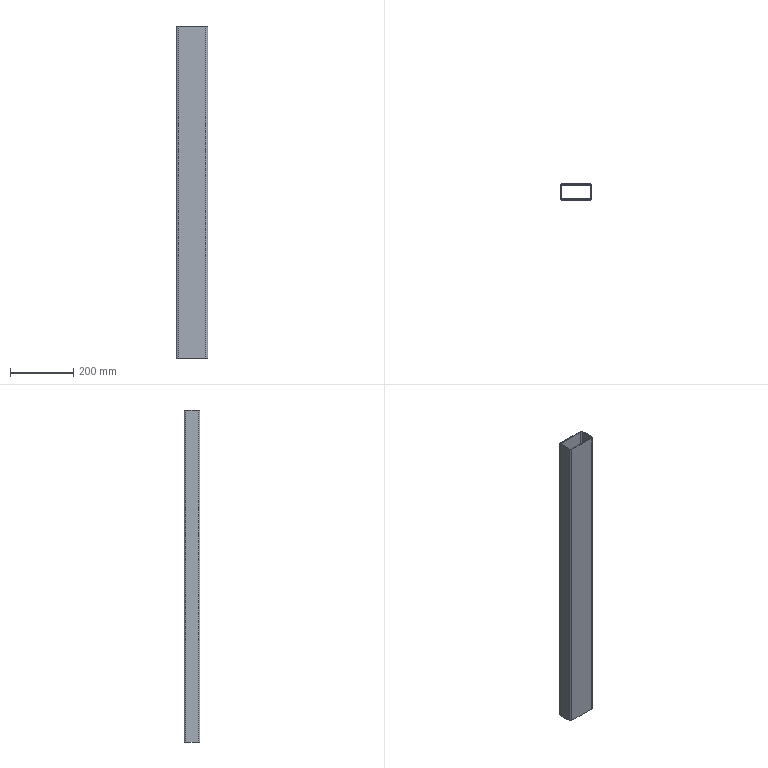Part | SolidWorks | features BaseBody 1 | 1 solid | 18 faces | box 100 x 50 x 1046 mm | volume 879501 mm3 | plane 10 | cylinder 8 | commonest cylinder face diameters 6 x4 12 x4
STEP:
#1=CARTESIAN_POINT('',(-44.,-22.,0.));
#2=VERTEX_POINT('',#1);
#3=CARTESIAN_POINT('',(44.,-22.,0.));
#4=VERTEX_POINT('',#3);
#5=CARTESIAN_POINT('',(44.,-22.,0.));
#6=DIRECTION('',(1.,0.,0.));
#7=VECTOR('',#6,1000.);
#8=LINE('',#5,#7);
#9=EDGE_CURVE('',#2,#4,#8,.T.);
#10=ORIENTED_EDGE('',*,*,#9,.F.);
#11=CARTESIAN_POINT('',(-44.,-22.,1046.));
#12=VERTEX_POINT('',#11);
#13=CARTESIAN_POINT('',(-44.,-22.,1046.));
#14=DIRECTION('',(0.,0.,-1.));
#15=VECTOR('',#14,1000.);
#16=LINE('',#13,#15);
#17=EDGE_CURVE('',#12,#2,#16,.T.);
#18=ORIENTED_EDGE('',*,*,#17,.F.);
#19=CARTESIAN_POINT('',(44.,-22.,1046.));
#20=VERTEX_POINT('',#19);
#21=CARTESIAN_POINT('',(44.,-22.,1046.));
#22=DIRECTION('',(1.,0.,0.));
#23=VECTOR('',#22,1000.);
#24=LINE('',#21,#23);
#25=EDGE_CURVE('',#12,#20,#24,.T.);
#26=ORIENTED_EDGE('',*,*,#25,.T.);
#27=CARTESIAN_POINT('',(44.,-22.,1046.));
#28=DIRECTION('',(0.,0.,-1.));
#29=VECTOR('',#28,1000.);
#30=LINE('',#27,#29);
#31=EDGE_CURVE('',#20,#4,#30,.T.);
#32=ORIENTED_EDGE('',*,*,#31,.T.);
#33=EDGE_LOOP('',(#10,#18,#26,#32));
#34=FACE_OUTER_BOUND('',#33,.T.);
#35=CARTESIAN_POINT('',(44.,-22.,1046.));
#36=DIRECTION('',(0.,1.,0.));
#37=DIRECTION('',(1.,0.,0.));
#38=AXIS2_PLACEMENT_3D('',#35,#36,#37);
#39=PLANE('',#38);
#40=ADVANCED_FACE('',(#34),#39,.T.);
#41=CARTESIAN_POINT('',(-47.,-19.,0.));
#42=VERTEX_POINT('',#41);
#43=CARTESIAN_POINT('',(-44.,-19.,0.));
#44=DIRECTION('',(0.,0.,1.));
#45=DIRECTION('',(-1.,0.,0.));
#46=AXIS2_PLACEMENT_3D('',#43,#44,#45);
#47=CIRCLE('',#46,3.);
#48=EDGE_CURVE('',#42,#2,#47,.T.);
#49=ORIENTED_EDGE('',*,*,#48,.F.);
#50=CARTESIAN_POINT('',(-47.,-19.,1046.));
#51=VERTEX_POINT('',#50);
#52=CARTESIAN_POINT('',(-47.,-19.,1046.));
#53=DIRECTION('',(0.,0.,-1.));
#54=VECTOR('',#53,1000.);
#55=LINE('',#52,#54);
#56=EDGE_CURVE('',#51,#42,#55,.T.);
#57=ORIENTED_EDGE('',*,*,#56,.F.);
#58=CARTESIAN_POINT('',(-44.,-19.,1046.));
#59=DIRECTION('',(0.,0.,1.));
#60=DIRECTION('',(-1.,0.,0.));
#61=AXIS2_PLACEMENT_3D('',#58,#59,#60);
#62=CIRCLE('',#61,3.);
#63=EDGE_CURVE('',#51,#12,#62,.T.);
#64=ORIENTED_EDGE('',*,*,#63,.T.);
#65=ORIENTED_EDGE('',*,*,#17,.T.);
#66=EDGE_LOOP('',(#49,#57,#64,#65));
#67=FACE_OUTER_BOUND('',#66,.T.);
#68=CARTESIAN_POINT('',(-44.,-19.,1046.));
#69=DIRECTION('',(0.,0.,-1.));
#70=DIRECTION('',(-1.,0.,0.));
#71=AXIS2_PLACEMENT_3D('',#68,#69,#70);
#72=CYLINDRICAL_SURFACE('',#71,3.);
#73=ADVANCED_FACE('',(#67),#72,.F.);
#74=CARTESIAN_POINT('',(-47.,19.,0.));
#75=VERTEX_POINT('',#74);
#76=CARTESIAN_POINT('',(-47.,19.,0.));
#77=DIRECTION('',(0.,-1.,0.));
#78=VECTOR('',#77,1000.);
#79=LINE('',#76,#78);
#80=EDGE_CURVE('',#75,#42,#79,.T.);
#81=ORIENTED_EDGE('',*,*,#80,.F.);
#82=CARTESIAN_POINT('',(-47.,19.,1046.));
#83=VERTEX_POINT('',#82);
#84=CARTESIAN_POINT('',(-47.,19.,1046.));
#85=DIRECTION('',(0.,0.,-1.));
#86=VECTOR('',#85,1000.);
#87=LINE('',#84,#86);
#88=EDGE_CURVE('',#83,#75,#87,.T.);
#89=ORIENTED_EDGE('',*,*,#88,.F.);
#90=CARTESIAN_POINT('',(-47.,19.,1046.));
#91=DIRECTION('',(0.,-1.,0.));
#92=VECTOR('',#91,1000.);
#93=LINE('',#90,#92);
#94=EDGE_CURVE('',#83,#51,#93,.T.);
#95=ORIENTED_EDGE('',*,*,#94,.T.);
#96=ORIENTED_EDGE('',*,*,#56,.T.);
#97=EDGE_LOOP('',(#81,#89,#95,#96));
#98=FACE_OUTER_BOUND('',#97,.T.);
#99=CARTESIAN_POINT('',(-47.,19.,1046.));
#100=DIRECTION('',(1.,0.,0.));
#101=DIRECTION('',(0.,1.,0.));
#102=AXIS2_PLACEMENT_3D('',#99,#100,#101);
#103=PLANE('',#102);
#104=ADVANCED_FACE('',(#98),#103,.T.);
#105=CARTESIAN_POINT('',(-44.,22.,0.));
#106=VERTEX_POINT('',#105);
#107=CARTESIAN_POINT('',(-44.,19.,0.));
#108=DIRECTION('',(0.,0.,1.));
#109=DIRECTION('',(-1.,0.,0.));
#110=AXIS2_PLACEMENT_3D('',#107,#108,#109);
#111=CIRCLE('',#110,3.);
#112=EDGE_CURVE('',#106,#75,#111,.T.);
#113=ORIENTED_EDGE('',*,*,#112,.F.);
#114=CARTESIAN_POINT('',(-44.,22.,1046.));
#115=VERTEX_POINT('',#114);
#116=CARTESIAN_POINT('',(-44.,22.,1046.));
#117=DIRECTION('',(0.,0.,-1.));
#118=VECTOR('',#117,1000.);
#119=LINE('',#116,#118);
#120=EDGE_CURVE('',#115,#106,#119,.T.);
#121=ORIENTED_EDGE('',*,*,#120,.F.);
#122=CARTESIAN_POINT('',(-44.,19.,1046.));
#123=DIRECTION('',(0.,0.,1.));
#124=DIRECTION('',(-1.,0.,0.));
#125=AXIS2_PLACEMENT_3D('',#122,#123,#124);
#126=CIRCLE('',#125,3.);
#127=EDGE_CURVE('',#115,#83,#126,.T.);
#128=ORIENTED_EDGE('',*,*,#127,.T.);
#129=ORIENTED_EDGE('',*,*,#88,.T.);
#130=EDGE_LOOP('',(#113,#121,#128,#129));
#131=FACE_OUTER_BOUND('',#130,.T.);
#132=CARTESIAN_POINT('',(-44.,19.,1046.));
#133=DIRECTION('',(0.,0.,-1.));
#134=DIRECTION('',(-1.,0.,0.));
#135=AXIS2_PLACEMENT_3D('',#132,#133,#134);
#136=CYLINDRICAL_SURFACE('',#135,3.);
#137=ADVANCED_FACE('',(#131),#136,.F.);
#138=CARTESIAN_POINT('',(44.,22.,0.));
#139=VERTEX_POINT('',#138);
#140=CARTESIAN_POINT('',(44.,22.,0.));
#141=DIRECTION('',(-1.,0.,0.));
#142=VECTOR('',#141,1000.);
#143=LINE('',#140,#142);
#144=EDGE_CURVE('',#139,#106,#143,.T.);
#145=ORIENTED_EDGE('',*,*,#144,.F.);
#146=CARTESIAN_POINT('',(44.,22.,1046.));
#147=VERTEX_POINT('',#146);
#148=CARTESIAN_POINT('',(44.,22.,1046.));
#149=DIRECTION('',(0.,0.,-1.));
#150=VECTOR('',#149,1000.);
#151=LINE('',#148,#150);
#152=EDGE_CURVE('',#147,#139,#151,.T.);
#153=ORIENTED_EDGE('',*,*,#152,.F.);
#154=CARTESIAN_POINT('',(44.,22.,1046.));
#155=DIRECTION('',(-1.,0.,0.));
#156=VECTOR('',#155,1000.);
#157=LINE('',#154,#156);
#158=EDGE_CURVE('',#147,#115,#157,.T.);
#159=ORIENTED_EDGE('',*,*,#158,.T.);
#160=ORIENTED_EDGE('',*,*,#120,.T.);
#161=EDGE_LOOP('',(#145,#153,#159,#160));
#162=FACE_OUTER_BOUND('',#161,.T.);
#163=CARTESIAN_POINT('',(44.,22.,1046.));
#164=DIRECTION('',(0.,-1.,0.));
#165=DIRECTION('',(0.,0.,-1.));
#166=AXIS2_PLACEMENT_3D('',#163,#164,#165);
#167=PLANE('',#166);
#168=ADVANCED_FACE('',(#162),#167,.T.);
#169=CARTESIAN_POINT('',(47.,19.,0.));
#170=VERTEX_POINT('',#169);
#171=CARTESIAN_POINT('',(44.,19.,0.));
#172=DIRECTION('',(0.,0.,1.));
#173=DIRECTION('',(1.,0.,0.));
#174=AXIS2_PLACEMENT_3D('',#171,#172,#173);
#175=CIRCLE('',#174,3.);
#176=EDGE_CURVE('',#170,#139,#175,.T.);
#177=ORIENTED_EDGE('',*,*,#176,.F.);
#178=CARTESIAN_POINT('',(47.,19.,1046.));
#179=VERTEX_POINT('',#178);
#180=CARTESIAN_POINT('',(47.,19.,1046.));
#181=DIRECTION('',(0.,0.,-1.));
#182=VECTOR('',#181,1000.);
#183=LINE('',#180,#182);
#184=EDGE_CURVE('',#179,#170,#183,.T.);
#185=ORIENTED_EDGE('',*,*,#184,.F.);
#186=CARTESIAN_POINT('',(44.,19.,1046.));
#187=DIRECTION('',(0.,0.,1.));
#188=DIRECTION('',(1.,0.,0.));
#189=AXIS2_PLACEMENT_3D('',#186,#187,#188);
#190=CIRCLE('',#189,3.);
#191=EDGE_CURVE('',#179,#147,#190,.T.);
#192=ORIENTED_EDGE('',*,*,#191,.T.);
#193=ORIENTED_EDGE('',*,*,#152,.T.);
#194=EDGE_LOOP('',(#177,#185,#192,#193));
#195=FACE_OUTER_BOUND('',#194,.T.);
#196=CARTESIAN_POINT('',(44.,19.,1046.));
#197=DIRECTION('',(0.,0.,-1.));
#198=DIRECTION('',(-1.,0.,0.));
#199=AXIS2_PLACEMENT_3D('',#196,#197,#198);
#200=CYLINDRICAL_SURFACE('',#199,3.);
#201=ADVANCED_FACE('',(#195),#200,.F.);
#202=CARTESIAN_POINT('',(47.,-19.,0.));
#203=VERTEX_POINT('',#202);
#204=CARTESIAN_POINT('',(47.,19.,0.));
#205=DIRECTION('',(0.,1.,0.));
#206=VECTOR('',#205,1000.);
#207=LINE('',#204,#206);
#208=EDGE_CURVE('',#203,#170,#207,.T.);
#209=ORIENTED_EDGE('',*,*,#208,.F.);
#210=CARTESIAN_POINT('',(47.,-19.,1046.));
#211=VERTEX_POINT('',#210);
#212=CARTESIAN_POINT('',(47.,-19.,1046.));
#213=DIRECTION('',(0.,0.,-1.));
#214=VECTOR('',#213,1000.);
#215=LINE('',#212,#214);
#216=EDGE_CURVE('',#211,#203,#215,.T.);
#217=ORIENTED_EDGE('',*,*,#216,.F.);
#218=CARTESIAN_POINT('',(47.,19.,1046.));
#219=DIRECTION('',(0.,1.,0.));
#220=VECTOR('',#219,1000.);
#221=LINE('',#218,#220);
#222=EDGE_CURVE('',#211,#179,#221,.T.);
#223=ORIENTED_EDGE('',*,*,#222,.T.);
#224=ORIENTED_EDGE('',*,*,#184,.T.);
#225=EDGE_LOOP('',(#209,#217,#223,#224));
#226=FACE_OUTER_BOUND('',#225,.T.);
#227=CARTESIAN_POINT('',(47.,19.,1046.));
#228=DIRECTION('',(-1.,0.,0.));
#229=DIRECTION('',(0.,0.,1.));
#230=AXIS2_PLACEMENT_3D('',#227,#228,#229);
#231=PLANE('',#230);
#232=ADVANCED_FACE('',(#226),#231,.T.);
#233=CARTESIAN_POINT('',(44.,-19.,0.));
#234=DIRECTION('',(0.,0.,1.));
#235=DIRECTION('',(-1.,0.,0.));
#236=AXIS2_PLACEMENT_3D('',#233,#234,#235);
#237=CIRCLE('',#236,3.);
#238=EDGE_CURVE('',#4,#203,#237,.T.);
#239=ORIENTED_EDGE('',*,*,#238,.F.);
#240=ORIENTED_EDGE('',*,*,#31,.F.);
#241=CARTESIAN_POINT('',(44.,-19.,1046.));
#242=DIRECTION('',(0.,0.,1.));
#243=DIRECTION('',(-1.,0.,0.));
#244=AXIS2_PLACEMENT_3D('',#241,#242,#243);
#245=CIRCLE('',#244,3.);
#246=EDGE_CURVE('',#20,#211,#245,.T.);
#247=ORIENTED_EDGE('',*,*,#246,.T.);
#248=ORIENTED_EDGE('',*,*,#216,.T.);
#249=EDGE_LOOP('',(#239,#240,#247,#248));
#250=FACE_OUTER_BOUND('',#249,.T.);
#251=CARTESIAN_POINT('',(44.,-19.,1046.));
#252=DIRECTION('',(0.,0.,-1.));
#253=DIRECTION('',(-1.,0.,0.));
#254=AXIS2_PLACEMENT_3D('',#251,#252,#253);
#255=CYLINDRICAL_SURFACE('',#254,3.);
#256=ADVANCED_FACE('',(#250),#255,.F.);
#257=CARTESIAN_POINT('',(50.,-19.,0.));
#258=VERTEX_POINT('',#257);
#259=CARTESIAN_POINT('',(50.,19.,0.));
#260=VERTEX_POINT('',#259);
#261=CARTESIAN_POINT('',(50.,19.,0.));
#262=DIRECTION('',(0.,1.,0.));
#263=VECTOR('',#262,1000.);
#264=LINE('',#261,#263);
#265=EDGE_CURVE('',#258,#260,#264,.T.);
#266=ORIENTED_EDGE('',*,*,#265,.T.);
#267=CARTESIAN_POINT('',(50.,19.,1046.));
#268=VERTEX_POINT('',#267);
#269=CARTESIAN_POINT('',(50.,19.,1046.));
#270=DIRECTION('',(0.,0.,-1.));
#271=VECTOR('',#270,1000.);
#272=LINE('',#269,#271);
#273=EDGE_CURVE('',#268,#260,#272,.T.);
#274=ORIENTED_EDGE('',*,*,#273,.F.);
#275=CARTESIAN_POINT('',(50.,-19.,1046.));
#276=VERTEX_POINT('',#275);
#277=CARTESIAN_POINT('',(50.,19.,1046.));
#278=DIRECTION('',(0.,1.,0.));
#279=VECTOR('',#278,1000.);
#280=LINE('',#277,#279);
#281=EDGE_CURVE('',#276,#268,#280,.T.);
#282=ORIENTED_EDGE('',*,*,#281,.F.);
#283=CARTESIAN_POINT('',(50.,-19.,1046.));
#284=DIRECTION('',(0.,0.,-1.));
#285=VECTOR('',#284,1000.);
#286=LINE('',#283,#285);
#287=EDGE_CURVE('',#276,#258,#286,.T.);
#288=ORIENTED_EDGE('',*,*,#287,.T.);
#289=EDGE_LOOP('',(#266,#274,#282,#288));
#290=FACE_OUTER_BOUND('',#289,.T.);
#291=CARTESIAN_POINT('',(50.,19.,1046.));
#292=DIRECTION('',(-1.,0.,0.));
#293=DIRECTION('',(0.,1.,0.));
#294=AXIS2_PLACEMENT_3D('',#291,#292,#293);
#295=PLANE('',#294);
#296=ADVANCED_FACE('',(#290),#295,.F.);
#297=CARTESIAN_POINT('',(44.,-25.,0.));
#298=VERTEX_POINT('',#297);
#299=CARTESIAN_POINT('',(44.,-19.,0.));
#300=DIRECTION('',(0.,0.,1.));
#301=DIRECTION('',(-1.,0.,0.));
#302=AXIS2_PLACEMENT_3D('',#299,#300,#301);
#303=CIRCLE('',#302,6.);
#304=EDGE_CURVE('',#298,#258,#303,.T.);
#305=ORIENTED_EDGE('',*,*,#304,.T.);
#306=ORIENTED_EDGE('',*,*,#287,.F.);
#307=CARTESIAN_POINT('',(44.,-25.,1046.));
#308=VERTEX_POINT('',#307);
#309=CARTESIAN_POINT('',(44.,-19.,1046.));
#310=DIRECTION('',(0.,0.,1.));
#311=DIRECTION('',(-1.,0.,0.));
#312=AXIS2_PLACEMENT_3D('',#309,#310,#311);
#313=CIRCLE('',#312,6.);
#314=EDGE_CURVE('',#308,#276,#313,.T.);
#315=ORIENTED_EDGE('',*,*,#314,.F.);
#316=CARTESIAN_POINT('',(44.,-25.,1046.));
#317=DIRECTION('',(0.,0.,-1.));
#318=VECTOR('',#317,1000.);
#319=LINE('',#316,#318);
#320=EDGE_CURVE('',#308,#298,#319,.T.);
#321=ORIENTED_EDGE('',*,*,#320,.T.);
#322=EDGE_LOOP('',(#305,#306,#315,#321));
#323=FACE_OUTER_BOUND('',#322,.T.);
#324=CARTESIAN_POINT('',(44.,-19.,1046.));
#325=DIRECTION('',(0.,0.,-1.));
#326=DIRECTION('',(-1.,0.,0.));
#327=AXIS2_PLACEMENT_3D('',#324,#325,#326);
#328=CYLINDRICAL_SURFACE('',#327,6.);
#329=ADVANCED_FACE('',(#323),#328,.T.);
#330=CARTESIAN_POINT('',(-44.,-25.,0.));
#331=VERTEX_POINT('',#330);
#332=CARTESIAN_POINT('',(44.,-25.,0.));
#333=DIRECTION('',(1.,0.,0.));
#334=VECTOR('',#333,1000.);
#335=LINE('',#332,#334);
#336=EDGE_CURVE('',#331,#298,#335,.T.);
#337=ORIENTED_EDGE('',*,*,#336,.T.);
#338=ORIENTED_EDGE('',*,*,#320,.F.);
#339=CARTESIAN_POINT('',(-44.,-25.,1046.));
#340=VERTEX_POINT('',#339);
#341=CARTESIAN_POINT('',(44.,-25.,1046.));
#342=DIRECTION('',(1.,0.,0.));
#343=VECTOR('',#342,1000.);
#344=LINE('',#341,#343);
#345=EDGE_CURVE('',#340,#308,#344,.T.);
#346=ORIENTED_EDGE('',*,*,#345,.F.);
#347=CARTESIAN_POINT('',(-44.,-25.,1046.));
#348=DIRECTION('',(0.,0.,-1.));
#349=VECTOR('',#348,1000.);
#350=LINE('',#347,#349);
#351=EDGE_CURVE('',#340,#331,#350,.T.);
#352=ORIENTED_EDGE('',*,*,#351,.T.);
#353=EDGE_LOOP('',(#337,#338,#346,#352));
#354=FACE_OUTER_BOUND('',#353,.T.);
#355=CARTESIAN_POINT('',(44.,-25.,1046.));
#356=DIRECTION('',(0.,1.,0.));
#357=DIRECTION('',(1.,0.,0.));
#358=AXIS2_PLACEMENT_3D('',#355,#356,#357);
#359=PLANE('',#358);
#360=ADVANCED_FACE('',(#354),#359,.F.);
#361=CARTESIAN_POINT('',(-50.,-19.,0.));
#362=VERTEX_POINT('',#361);
#363=CARTESIAN_POINT('',(-44.,-19.,0.));
#364=DIRECTION('',(0.,0.,1.));
#365=DIRECTION('',(-1.,0.,0.));
#366=AXIS2_PLACEMENT_3D('',#363,#364,#365);
#367=CIRCLE('',#366,6.);
#368=EDGE_CURVE('',#362,#331,#367,.T.);
#369=ORIENTED_EDGE('',*,*,#368,.T.);
#370=ORIENTED_EDGE('',*,*,#351,.F.);
#371=CARTESIAN_POINT('',(-50.,-19.,1046.));
#372=VERTEX_POINT('',#371);
#373=CARTESIAN_POINT('',(-44.,-19.,1046.));
#374=DIRECTION('',(0.,0.,1.));
#375=DIRECTION('',(-1.,0.,0.));
#376=AXIS2_PLACEMENT_3D('',#373,#374,#375);
#377=CIRCLE('',#376,6.);
#378=EDGE_CURVE('',#372,#340,#377,.T.);
#379=ORIENTED_EDGE('',*,*,#378,.F.);
#380=CARTESIAN_POINT('',(-50.,-19.,1046.));
#381=DIRECTION('',(0.,0.,-1.));
#382=VECTOR('',#381,1000.);
#383=LINE('',#380,#382);
#384=EDGE_CURVE('',#372,#362,#383,.T.);
#385=ORIENTED_EDGE('',*,*,#384,.T.);
#386=EDGE_LOOP('',(#369,#370,#379,#385));
#387=FACE_OUTER_BOUND('',#386,.T.);
#388=CARTESIAN_POINT('',(-44.,-19.,1046.));
#389=DIRECTION('',(0.,0.,-1.));
#390=DIRECTION('',(-1.,0.,0.));
#391=AXIS2_PLACEMENT_3D('',#388,#389,#390);
#392=CYLINDRICAL_SURFACE('',#391,6.);
#393=ADVANCED_FACE('',(#387),#392,.T.);
#394=CARTESIAN_POINT('',(-50.,19.,0.));
#395=VERTEX_POINT('',#394);
#396=CARTESIAN_POINT('',(-50.,19.,0.));
#397=DIRECTION('',(0.,-1.,0.));
#398=VECTOR('',#397,1000.);
#399=LINE('',#396,#398);
#400=EDGE_CURVE('',#395,#362,#399,.T.);
#401=ORIENTED_EDGE('',*,*,#400,.T.);
#402=ORIENTED_EDGE('',*,*,#384,.F.);
#403=CARTESIAN_POINT('',(-50.,19.,1046.));
#404=VERTEX_POINT('',#403);
#405=CARTESIAN_POINT('',(-50.,19.,1046.));
#406=DIRECTION('',(0.,-1.,0.));
#407=VECTOR('',#406,1000.);
#408=LINE('',#405,#407);
#409=EDGE_CURVE('',#404,#372,#408,.T.);
#410=ORIENTED_EDGE('',*,*,#409,.F.);
#411=CARTESIAN_POINT('',(-50.,19.,1046.));
#412=DIRECTION('',(0.,0.,-1.));
#413=VECTOR('',#412,1000.);
#414=LINE('',#411,#413);
#415=EDGE_CURVE('',#404,#395,#414,.T.);
#416=ORIENTED_EDGE('',*,*,#415,.T.);
#417=EDGE_LOOP('',(#401,#402,#410,#416));
#418=FACE_OUTER_BOUND('',#417,.T.);
#419=CARTESIAN_POINT('',(-50.,19.,1046.));
#420=DIRECTION('',(1.,0.,0.));
#421=DIRECTION('',(0.,1.,0.));
#422=AXIS2_PLACEMENT_3D('',#419,#420,#421);
#423=PLANE('',#422);
#424=ADVANCED_FACE('',(#418),#423,.F.);
#425=CARTESIAN_POINT('',(-44.,25.,0.));
#426=VERTEX_POINT('',#425);
#427=CARTESIAN_POINT('',(-44.,19.,0.));
#428=DIRECTION('',(0.,0.,1.));
#429=DIRECTION('',(1.,0.,0.));
#430=AXIS2_PLACEMENT_3D('',#427,#428,#429);
#431=CIRCLE('',#430,6.);
#432=EDGE_CURVE('',#426,#395,#431,.T.);
#433=ORIENTED_EDGE('',*,*,#432,.T.);
#434=ORIENTED_EDGE('',*,*,#415,.F.);
#435=CARTESIAN_POINT('',(-44.,25.,1046.));
#436=VERTEX_POINT('',#435);
#437=CARTESIAN_POINT('',(-44.,19.,1046.));
#438=DIRECTION('',(0.,0.,1.));
#439=DIRECTION('',(1.,0.,0.));
#440=AXIS2_PLACEMENT_3D('',#437,#438,#439);
#441=CIRCLE('',#440,6.);
#442=EDGE_CURVE('',#436,#404,#441,.T.);
#443=ORIENTED_EDGE('',*,*,#442,.F.);
#444=CARTESIAN_POINT('',(-44.,25.,1046.));
#445=DIRECTION('',(0.,0.,-1.));
#446=VECTOR('',#445,1000.);
#447=LINE('',#444,#446);
#448=EDGE_CURVE('',#436,#426,#447,.T.);
#449=ORIENTED_EDGE('',*,*,#448,.T.);
#450=EDGE_LOOP('',(#433,#434,#443,#449));
#451=FACE_OUTER_BOUND('',#450,.T.);
#452=CARTESIAN_POINT('',(-44.,19.,1046.));
#453=DIRECTION('',(0.,0.,-1.));
#454=DIRECTION('',(-1.,0.,0.));
#455=AXIS2_PLACEMENT_3D('',#452,#453,#454);
#456=CYLINDRICAL_SURFACE('',#455,6.);
#457=ADVANCED_FACE('',(#451),#456,.T.);
#458=CARTESIAN_POINT('',(44.,25.,0.));
#459=VERTEX_POINT('',#458);
#460=CARTESIAN_POINT('',(44.,25.,0.));
#461=DIRECTION('',(-1.,0.,0.));
#462=VECTOR('',#461,1000.);
#463=LINE('',#460,#462);
#464=EDGE_CURVE('',#459,#426,#463,.T.);
#465=ORIENTED_EDGE('',*,*,#464,.T.);
#466=ORIENTED_EDGE('',*,*,#448,.F.);
#467=CARTESIAN_POINT('',(44.,25.,1046.));
#468=VERTEX_POINT('',#467);
#469=CARTESIAN_POINT('',(44.,25.,1046.));
#470=DIRECTION('',(-1.,0.,0.));
#471=VECTOR('',#470,1000.);
#472=LINE('',#469,#471);
#473=EDGE_CURVE('',#468,#436,#472,.T.);
#474=ORIENTED_EDGE('',*,*,#473,.F.);
#475=CARTESIAN_POINT('',(44.,25.,1046.));
#476=DIRECTION('',(0.,0.,-1.));
#477=VECTOR('',#476,1000.);
#478=LINE('',#475,#477);
#479=EDGE_CURVE('',#468,#459,#478,.T.);
#480=ORIENTED_EDGE('',*,*,#479,.T.);
#481=EDGE_LOOP('',(#465,#466,#474,#480));
#482=FACE_OUTER_BOUND('',#481,.T.);
#483=CARTESIAN_POINT('',(44.,25.,1046.));
#484=DIRECTION('',(0.,-1.,0.));
#485=DIRECTION('',(0.,0.,-1.));
#486=AXIS2_PLACEMENT_3D('',#483,#484,#485);
#487=PLANE('',#486);
#488=ADVANCED_FACE('',(#482),#487,.F.);
#489=CARTESIAN_POINT('',(44.,19.,0.));
#490=DIRECTION('',(0.,0.,1.));
#491=DIRECTION('',(-1.,0.,0.));
#492=AXIS2_PLACEMENT_3D('',#489,#490,#491);
#493=CIRCLE('',#492,6.);
#494=EDGE_CURVE('',#260,#459,#493,.T.);
#495=ORIENTED_EDGE('',*,*,#494,.T.);
#496=ORIENTED_EDGE('',*,*,#479,.F.);
#497=CARTESIAN_POINT('',(44.,19.,1046.));
#498=DIRECTION('',(0.,0.,1.));
#499=DIRECTION('',(-1.,0.,0.));
#500=AXIS2_PLACEMENT_3D('',#497,#498,#499);
#501=CIRCLE('',#500,6.);
#502=EDGE_CURVE('',#268,#468,#501,.T.);
#503=ORIENTED_EDGE('',*,*,#502,.F.);
#504=ORIENTED_EDGE('',*,*,#273,.T.);
#505=EDGE_LOOP('',(#495,#496,#503,#504));
#506=FACE_OUTER_BOUND('',#505,.T.);
#507=CARTESIAN_POINT('',(44.,19.,1046.));
#508=DIRECTION('',(0.,0.,-1.));
#509=DIRECTION('',(-1.,0.,0.));
#510=AXIS2_PLACEMENT_3D('',#507,#508,#509);
#511=CYLINDRICAL_SURFACE('',#510,6.);
#512=ADVANCED_FACE('',(#506),#511,.T.);
#513=ORIENTED_EDGE('',*,*,#9,.T.);
#514=ORIENTED_EDGE('',*,*,#238,.T.);
#515=ORIENTED_EDGE('',*,*,#208,.T.);
#516=ORIENTED_EDGE('',*,*,#176,.T.);
#517=ORIENTED_EDGE('',*,*,#144,.T.);
#518=ORIENTED_EDGE('',*,*,#112,.T.);
#519=ORIENTED_EDGE('',*,*,#80,.T.);
#520=ORIENTED_EDGE('',*,*,#48,.T.);
#521=EDGE_LOOP('',(#513,#514,#515,#516,#517,#518,#519,#520));
#522=FACE_BOUND('',#521,.T.);
#523=ORIENTED_EDGE('',*,*,#494,.F.);
#524=ORIENTED_EDGE('',*,*,#265,.F.);
#525=ORIENTED_EDGE('',*,*,#304,.F.);
#526=ORIENTED_EDGE('',*,*,#336,.F.);
#527=ORIENTED_EDGE('',*,*,#368,.F.);
#528=ORIENTED_EDGE('',*,*,#400,.F.);
#529=ORIENTED_EDGE('',*,*,#432,.F.);
#530=ORIENTED_EDGE('',*,*,#464,.F.);
#531=EDGE_LOOP('',(#523,#524,#525,#526,#527,#528,#529,#530));
#532=FACE_OUTER_BOUND('',#531,.T.);
#533=CARTESIAN_POINT('',(44.,19.,0.));
#534=DIRECTION('',(0.,0.,-1.));
#535=DIRECTION('',(0.,-1.,0.));
#536=AXIS2_PLACEMENT_3D('',#533,#534,#535);
#537=PLANE('',#536);
#538=ADVANCED_FACE('',(#522,#532),#537,.T.);
#539=ORIENTED_EDGE('',*,*,#246,.F.);
#540=ORIENTED_EDGE('',*,*,#25,.F.);
#541=ORIENTED_EDGE('',*,*,#63,.F.);
#542=ORIENTED_EDGE('',*,*,#94,.F.);
#543=ORIENTED_EDGE('',*,*,#127,.F.);
#544=ORIENTED_EDGE('',*,*,#158,.F.);
#545=ORIENTED_EDGE('',*,*,#191,.F.);
#546=ORIENTED_EDGE('',*,*,#222,.F.);
#547=EDGE_LOOP('',(#539,#540,#541,#542,#543,#544,#545,#546));
#548=FACE_BOUND('',#547,.T.);
#549=ORIENTED_EDGE('',*,*,#502,.T.);
#550=ORIENTED_EDGE('',*,*,#473,.T.);
#551=ORIENTED_EDGE('',*,*,#442,.T.);
#552=ORIENTED_EDGE('',*,*,#409,.T.);
#553=ORIENTED_EDGE('',*,*,#378,.T.);
#554=ORIENTED_EDGE('',*,*,#345,.T.);
#555=ORIENTED_EDGE('',*,*,#314,.T.);
#556=ORIENTED_EDGE('',*,*,#281,.T.);
#557=EDGE_LOOP('',(#549,#550,#551,#552,#553,#554,#555,#556));
#558=FACE_OUTER_BOUND('',#557,.T.);
#559=CARTESIAN_POINT('',(44.,19.,1046.));
#560=DIRECTION('',(0.,0.,-1.));
#561=DIRECTION('',(0.,-1.,0.));
#562=AXIS2_PLACEMENT_3D('',#559,#560,#561);
#563=PLANE('',#562);
#564=ADVANCED_FACE('',(#548,#558),#563,.F.);
#565=CLOSED_SHELL('',(#40,#73,#104,#137,#168,#201,#232,#256,#296,#329,#360,#393,#424,#457,#488,#512,#538,#564));
#566=MANIFOLD_SOLID_BREP('',#565);
#567=CARTESIAN_POINT('',(0.,0.,0.));
#568=DIRECTION('',(0.,0.,1.));
#569=DIRECTION('',(1.,0.,0.));
#570=AXIS2_PLACEMENT_3D('',#567,#568,#569);
#571=(LENGTH_UNIT()NAMED_UNIT(*)SI_UNIT(.MILLI.,.METRE.));
#572=UNCERTAINTY_MEASURE_WITH_UNIT(LENGTH_MEASURE(0.00001),#571,'','');
#573=(NAMED_UNIT(*)PLANE_ANGLE_UNIT()SI_UNIT($,.RADIAN.));
#574=(NAMED_UNIT(*)SI_UNIT($,.STERADIAN.)SOLID_ANGLE_UNIT());
#575=(GEOMETRIC_REPRESENTATION_CONTEXT(3)GLOBAL_UNCERTAINTY_ASSIGNED_CONTEXT((#572))GLOBAL_UNIT_ASSIGNED_CONTEXT((#571,#573,#574))REPRESENTATION_CONTEXT('',''));
#576=ADVANCED_BREP_SHAPE_REPRESENTATION('',(#566,#570),#575);